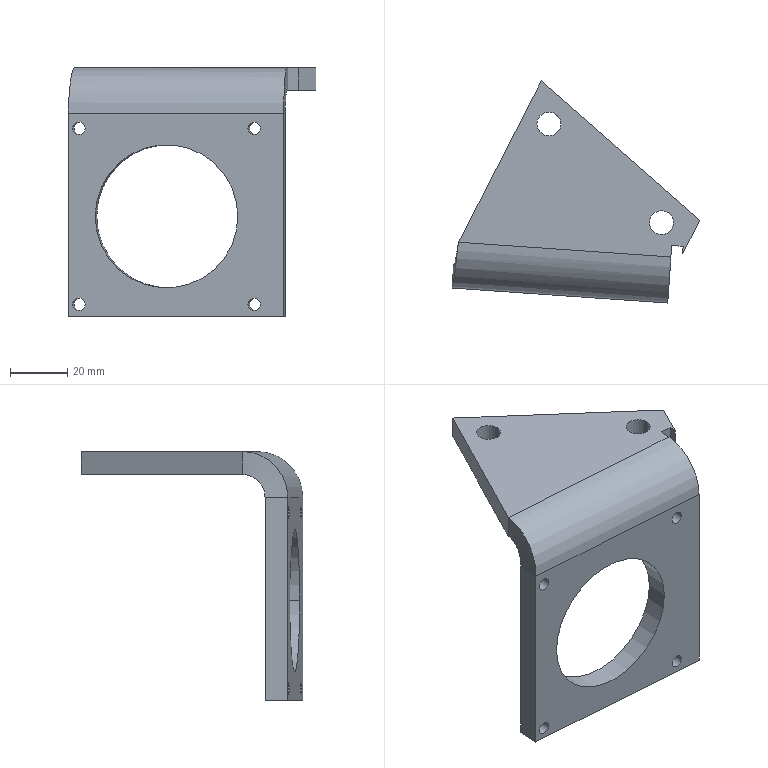Part | SolidWorks | features Cut 1, EdgeFlange 1, FlatPattern 1, ICE 1, SMBaseFlange 1, SheetMetal 1 | 1 solid | 31 faces | box 86.705 x 77.475 x 87.001 mm | volume 59436 mm3 | cylinder 16 | plane 14 | spline 1 | commonest cylinder face diameters 4.4 x8 8.382 x2 8.4 x2 50 x2 16 x1 32 x1
STEP:
#1=CARTESIAN_POINT('',(-134.069,-149.706,-52.));
#2=VERTEX_POINT('',#1);
#3=CARTESIAN_POINT('',(-183.95,-146.258,-52.));
#4=VERTEX_POINT('',#3);
#5=CARTESIAN_POINT('',(-159.009,-147.982,-52.));
#6=DIRECTION('',(0.06897,0.9976,0.));
#7=DIRECTION('',(-0.9976,0.06897,0.));
#8=AXIS2_PLACEMENT_3D('',#5,#6,#7);
#9=CIRCLE('',#8,25.);
#10=EDGE_CURVE('',#2,#4,#9,.T.);
#11=ORIENTED_EDGE('',*,*,#10,.F.);
#12=CARTESIAN_POINT('',(-133.517,-141.725,-52.));
#13=VERTEX_POINT('',#12);
#14=CARTESIAN_POINT('',(-134.207,-151.701,-52.));
#15=DIRECTION('',(0.06897,0.9976,0.));
#16=VECTOR('',#15,1000.);
#17=LINE('',#14,#16);
#18=EDGE_CURVE('',#2,#13,#17,.T.);
#19=ORIENTED_EDGE('',*,*,#18,.T.);
#20=CARTESIAN_POINT('',(-183.398,-138.277,-52.));
#21=VERTEX_POINT('',#20);
#22=CARTESIAN_POINT('',(-158.458,-140.001,-52.));
#23=DIRECTION('',(0.06897,0.9976,0.));
#24=DIRECTION('',(-0.9976,0.06897,0.));
#25=AXIS2_PLACEMENT_3D('',#22,#23,#24);
#26=CIRCLE('',#25,25.);
#27=EDGE_CURVE('',#13,#21,#26,.T.);
#28=ORIENTED_EDGE('',*,*,#27,.T.);
#29=CARTESIAN_POINT('',(-184.088,-148.253,-52.));
#30=DIRECTION('',(0.06897,0.9976,0.));
#31=VECTOR('',#30,1000.);
#32=LINE('',#29,#31);
#33=EDGE_CURVE('',#4,#21,#32,.T.);
#34=ORIENTED_EDGE('',*,*,#33,.F.);
#35=EDGE_LOOP('',(#11,#19,#28,#34));
#36=FACE_OUTER_BOUND('',#35,.T.);
#37=CARTESIAN_POINT('',(-159.147,-149.977,-52.));
#38=DIRECTION('',(0.06897,0.9976,0.));
#39=DIRECTION('',(-0.9976,0.06897,0.));
#40=AXIS2_PLACEMENT_3D('',#37,#38,#39);
#41=CYLINDRICAL_SURFACE('',#40,25.);
#42=ADVANCED_FACE('',(#36),#41,.F.);
#43=CARTESIAN_POINT('',(-126.136,-150.255,-82.75));
#44=VERTEX_POINT('',#43);
#45=CARTESIAN_POINT('',(-130.525,-149.951,-82.75));
#46=VERTEX_POINT('',#45);
#47=CARTESIAN_POINT('',(-128.33,-150.103,-82.75));
#48=DIRECTION('',(0.06897,0.9976,0.));
#49=DIRECTION('',(-0.9976,0.06897,0.));
#50=AXIS2_PLACEMENT_3D('',#47,#48,#49);
#51=CIRCLE('',#50,2.2);
#52=EDGE_CURVE('',#44,#46,#51,.T.);
#53=ORIENTED_EDGE('',*,*,#52,.F.);
#54=CARTESIAN_POINT('',(-125.584,-142.274,-82.75));
#55=VERTEX_POINT('',#54);
#56=CARTESIAN_POINT('',(-128.515,-184.673,-82.75));
#57=DIRECTION('',(0.06897,0.9976,0.));
#58=VECTOR('',#57,1000.);
#59=LINE('',#56,#58);
#60=EDGE_CURVE('',#44,#55,#59,.T.);
#61=ORIENTED_EDGE('',*,*,#60,.T.);
#62=CARTESIAN_POINT('',(-129.973,-141.97,-82.75));
#63=VERTEX_POINT('',#62);
#64=CARTESIAN_POINT('',(-127.779,-142.122,-82.75));
#65=DIRECTION('',(0.06897,0.9976,0.));
#66=DIRECTION('',(-0.9976,0.06897,0.));
#67=AXIS2_PLACEMENT_3D('',#64,#65,#66);
#68=CIRCLE('',#67,2.2);
#69=EDGE_CURVE('',#55,#63,#68,.T.);
#70=ORIENTED_EDGE('',*,*,#69,.T.);
#71=CARTESIAN_POINT('',(-132.905,-184.369,-82.75));
#72=DIRECTION('',(0.06897,0.9976,0.));
#73=VECTOR('',#72,1000.);
#74=LINE('',#71,#73);
#75=EDGE_CURVE('',#46,#63,#74,.T.);
#76=ORIENTED_EDGE('',*,*,#75,.F.);
#77=EDGE_LOOP('',(#53,#61,#70,#76));
#78=FACE_OUTER_BOUND('',#77,.T.);
#79=CARTESIAN_POINT('',(-130.71,-184.521,-82.75));
#80=DIRECTION('',(0.06897,0.9976,0.));
#81=DIRECTION('',(-0.9976,0.06897,0.));
#82=AXIS2_PLACEMENT_3D('',#79,#80,#81);
#83=CYLINDRICAL_SURFACE('',#82,2.2);
#84=ADVANCED_FACE('',(#78),#83,.F.);
#85=CARTESIAN_POINT('',(-187.489,-146.013,-82.75));
#86=VERTEX_POINT('',#85);
#87=CARTESIAN_POINT('',(-191.879,-145.709,-82.75));
#88=VERTEX_POINT('',#87);
#89=CARTESIAN_POINT('',(-189.684,-145.861,-82.75));
#90=DIRECTION('',(0.06897,0.9976,0.));
#91=DIRECTION('',(-0.9976,0.06897,0.));
#92=AXIS2_PLACEMENT_3D('',#89,#90,#91);
#93=CIRCLE('',#92,2.2);
#94=EDGE_CURVE('',#86,#88,#93,.T.);
#95=ORIENTED_EDGE('',*,*,#94,.F.);
#96=CARTESIAN_POINT('',(-186.937,-138.032,-82.75));
#97=VERTEX_POINT('',#96);
#98=CARTESIAN_POINT('',(-189.869,-180.431,-82.75));
#99=DIRECTION('',(0.06897,0.9976,0.));
#100=VECTOR('',#99,1000.);
#101=LINE('',#98,#100);
#102=EDGE_CURVE('',#86,#97,#101,.T.);
#103=ORIENTED_EDGE('',*,*,#102,.T.);
#104=CARTESIAN_POINT('',(-191.327,-137.729,-82.75));
#105=VERTEX_POINT('',#104);
#106=CARTESIAN_POINT('',(-189.132,-137.88,-82.75));
#107=DIRECTION('',(0.06897,0.9976,0.));
#108=DIRECTION('',(-0.9976,0.06897,0.));
#109=AXIS2_PLACEMENT_3D('',#106,#107,#108);
#110=CIRCLE('',#109,2.2);
#111=EDGE_CURVE('',#97,#105,#110,.T.);
#112=ORIENTED_EDGE('',*,*,#111,.T.);
#113=CARTESIAN_POINT('',(-194.258,-180.127,-82.75));
#114=DIRECTION('',(0.06897,0.9976,0.));
#115=VECTOR('',#114,1000.);
#116=LINE('',#113,#115);
#117=EDGE_CURVE('',#88,#105,#116,.T.);
#118=ORIENTED_EDGE('',*,*,#117,.F.);
#119=EDGE_LOOP('',(#95,#103,#112,#118));
#120=FACE_OUTER_BOUND('',#119,.T.);
#121=CARTESIAN_POINT('',(-192.063,-180.279,-82.75));
#122=DIRECTION('',(0.06897,0.9976,0.));
#123=DIRECTION('',(-0.9976,0.06897,0.));
#124=AXIS2_PLACEMENT_3D('',#121,#122,#123);
#125=CYLINDRICAL_SURFACE('',#124,2.2);
#126=ADVANCED_FACE('',(#120),#125,.F.);
#127=CARTESIAN_POINT('',(-187.489,-146.013,-21.25));
#128=VERTEX_POINT('',#127);
#129=CARTESIAN_POINT('',(-191.879,-145.709,-21.25));
#130=VERTEX_POINT('',#129);
#131=CARTESIAN_POINT('',(-189.684,-145.861,-21.25));
#132=DIRECTION('',(0.06897,0.9976,0.));
#133=DIRECTION('',(-0.9976,0.06897,0.));
#134=AXIS2_PLACEMENT_3D('',#131,#132,#133);
#135=CIRCLE('',#134,2.2);
#136=EDGE_CURVE('',#128,#130,#135,.T.);
#137=ORIENTED_EDGE('',*,*,#136,.F.);
#138=CARTESIAN_POINT('',(-186.937,-138.032,-21.25));
#139=VERTEX_POINT('',#138);
#140=CARTESIAN_POINT('',(-189.869,-180.431,-21.25));
#141=DIRECTION('',(0.06897,0.9976,0.));
#142=VECTOR('',#141,1000.);
#143=LINE('',#140,#142);
#144=EDGE_CURVE('',#128,#139,#143,.T.);
#145=ORIENTED_EDGE('',*,*,#144,.T.);
#146=CARTESIAN_POINT('',(-191.327,-137.729,-21.25));
#147=VERTEX_POINT('',#146);
#148=CARTESIAN_POINT('',(-189.132,-137.88,-21.25));
#149=DIRECTION('',(0.06897,0.9976,0.));
#150=DIRECTION('',(-0.9976,0.06897,0.));
#151=AXIS2_PLACEMENT_3D('',#148,#149,#150);
#152=CIRCLE('',#151,2.2);
#153=EDGE_CURVE('',#139,#147,#152,.T.);
#154=ORIENTED_EDGE('',*,*,#153,.T.);
#155=CARTESIAN_POINT('',(-194.258,-180.127,-21.25));
#156=DIRECTION('',(0.06897,0.9976,0.));
#157=VECTOR('',#156,1000.);
#158=LINE('',#155,#157);
#159=EDGE_CURVE('',#130,#147,#158,.T.);
#160=ORIENTED_EDGE('',*,*,#159,.F.);
#161=EDGE_LOOP('',(#137,#145,#154,#160));
#162=FACE_OUTER_BOUND('',#161,.T.);
#163=CARTESIAN_POINT('',(-192.063,-180.279,-21.25));
#164=DIRECTION('',(0.06897,0.9976,0.));
#165=DIRECTION('',(-0.9976,0.06897,0.));
#166=AXIS2_PLACEMENT_3D('',#163,#164,#165);
#167=CYLINDRICAL_SURFACE('',#166,2.2);
#168=ADVANCED_FACE('',(#162),#167,.F.);
#169=CARTESIAN_POINT('',(-126.136,-150.255,-21.25));
#170=VERTEX_POINT('',#169);
#171=CARTESIAN_POINT('',(-130.525,-149.951,-21.25));
#172=VERTEX_POINT('',#171);
#173=CARTESIAN_POINT('',(-128.33,-150.103,-21.25));
#174=DIRECTION('',(0.06897,0.9976,0.));
#175=DIRECTION('',(-0.9976,0.06897,0.));
#176=AXIS2_PLACEMENT_3D('',#173,#174,#175);
#177=CIRCLE('',#176,2.2);
#178=EDGE_CURVE('',#170,#172,#177,.T.);
#179=ORIENTED_EDGE('',*,*,#178,.F.);
#180=CARTESIAN_POINT('',(-125.584,-142.274,-21.25));
#181=VERTEX_POINT('',#180);
#182=CARTESIAN_POINT('',(-128.515,-184.673,-21.25));
#183=DIRECTION('',(0.06897,0.9976,0.));
#184=VECTOR('',#183,1000.);
#185=LINE('',#182,#184);
#186=EDGE_CURVE('',#170,#181,#185,.T.);
#187=ORIENTED_EDGE('',*,*,#186,.T.);
#188=CARTESIAN_POINT('',(-129.973,-141.97,-21.25));
#189=VERTEX_POINT('',#188);
#190=CARTESIAN_POINT('',(-127.779,-142.122,-21.25));
#191=DIRECTION('',(0.06897,0.9976,0.));
#192=DIRECTION('',(-0.9976,0.06897,0.));
#193=AXIS2_PLACEMENT_3D('',#190,#191,#192);
#194=CIRCLE('',#193,2.2);
#195=EDGE_CURVE('',#181,#189,#194,.T.);
#196=ORIENTED_EDGE('',*,*,#195,.T.);
#197=CARTESIAN_POINT('',(-132.905,-184.369,-21.25));
#198=DIRECTION('',(0.06897,0.9976,0.));
#199=VECTOR('',#198,1000.);
#200=LINE('',#197,#199);
#201=EDGE_CURVE('',#172,#189,#200,.T.);
#202=ORIENTED_EDGE('',*,*,#201,.F.);
#203=EDGE_LOOP('',(#179,#187,#196,#202));
#204=FACE_OUTER_BOUND('',#203,.T.);
#205=CARTESIAN_POINT('',(-130.71,-184.521,-21.25));
#206=DIRECTION('',(0.06897,0.9976,0.));
#207=DIRECTION('',(-0.9976,0.06897,0.));
#208=AXIS2_PLACEMENT_3D('',#205,#206,#207);
#209=CYLINDRICAL_SURFACE('',#208,2.2);
#210=ADVANCED_FACE('',(#204),#209,.F.);
#211=CARTESIAN_POINT('',(-124.39,-122.853,-8.));
#212=VERTEX_POINT('',#211);
#213=CARTESIAN_POINT('',(-115.99,-122.853,-8.));
#214=VERTEX_POINT('',#213);
#215=CARTESIAN_POINT('',(-120.19,-122.853,-8.));
#216=DIRECTION('',(0.,0.,1.));
#217=DIRECTION('',(-1.,0.,0.));
#218=AXIS2_PLACEMENT_3D('',#215,#216,#217);
#219=CIRCLE('',#218,4.2);
#220=EDGE_CURVE('',#212,#214,#219,.T.);
#221=ORIENTED_EDGE('',*,*,#220,.F.);
#222=CARTESIAN_POINT('',(-124.39,-122.853,0.));
#223=VERTEX_POINT('',#222);
#224=CARTESIAN_POINT('',(-124.39,-122.853,-8.));
#225=DIRECTION('',(0.,0.,1.));
#226=VECTOR('',#225,1000.);
#227=LINE('',#224,#226);
#228=EDGE_CURVE('',#212,#223,#227,.T.);
#229=ORIENTED_EDGE('',*,*,#228,.T.);
#230=CARTESIAN_POINT('',(-115.99,-122.853,0.));
#231=VERTEX_POINT('',#230);
#232=CARTESIAN_POINT('',(-120.19,-122.853,0.));
#233=DIRECTION('',(0.,0.,1.));
#234=DIRECTION('',(-1.,0.,0.));
#235=AXIS2_PLACEMENT_3D('',#232,#233,#234);
#236=CIRCLE('',#235,4.2);
#237=EDGE_CURVE('',#223,#231,#236,.T.);
#238=ORIENTED_EDGE('',*,*,#237,.T.);
#239=CARTESIAN_POINT('',(-115.99,-122.853,-8.));
#240=DIRECTION('',(0.,0.,1.));
#241=VECTOR('',#240,1000.);
#242=LINE('',#239,#241);
#243=EDGE_CURVE('',#214,#231,#242,.T.);
#244=ORIENTED_EDGE('',*,*,#243,.F.);
#245=EDGE_LOOP('',(#221,#229,#238,#244));
#246=FACE_OUTER_BOUND('',#245,.T.);
#247=CARTESIAN_POINT('',(-120.19,-122.853,-8.));
#248=DIRECTION('',(0.,0.,1.));
#249=DIRECTION('',(1.,0.,0.));
#250=AXIS2_PLACEMENT_3D('',#247,#248,#249);
#251=CYLINDRICAL_SURFACE('',#250,4.2);
#252=ADVANCED_FACE('',(#246),#251,.F.);
#253=CARTESIAN_POINT('',(-163.77,-88.351,-8.));
#254=VERTEX_POINT('',#253);
#255=CARTESIAN_POINT('',(-155.388,-88.351,-8.));
#256=VERTEX_POINT('',#255);
#257=CARTESIAN_POINT('',(-159.579,-88.351,-8.));
#258=DIRECTION('',(0.,0.,1.));
#259=DIRECTION('',(-1.,0.,0.));
#260=AXIS2_PLACEMENT_3D('',#257,#258,#259);
#261=CIRCLE('',#260,4.191);
#262=EDGE_CURVE('',#254,#256,#261,.T.);
#263=ORIENTED_EDGE('',*,*,#262,.F.);
#264=CARTESIAN_POINT('',(-163.77,-88.351,0.));
#265=VERTEX_POINT('',#264);
#266=CARTESIAN_POINT('',(-163.77,-88.351,-8.));
#267=DIRECTION('',(0.,0.,1.));
#268=VECTOR('',#267,1000.);
#269=LINE('',#266,#268);
#270=EDGE_CURVE('',#254,#265,#269,.T.);
#271=ORIENTED_EDGE('',*,*,#270,.T.);
#272=CARTESIAN_POINT('',(-155.388,-88.351,0.));
#273=VERTEX_POINT('',#272);
#274=CARTESIAN_POINT('',(-159.579,-88.351,0.));
#275=DIRECTION('',(0.,0.,1.));
#276=DIRECTION('',(-1.,0.,0.));
#277=AXIS2_PLACEMENT_3D('',#274,#275,#276);
#278=CIRCLE('',#277,4.191);
#279=EDGE_CURVE('',#265,#273,#278,.T.);
#280=ORIENTED_EDGE('',*,*,#279,.T.);
#281=CARTESIAN_POINT('',(-155.388,-88.351,-8.));
#282=DIRECTION('',(0.,0.,1.));
#283=VECTOR('',#282,1000.);
#284=LINE('',#281,#283);
#285=EDGE_CURVE('',#256,#273,#284,.T.);
#286=ORIENTED_EDGE('',*,*,#285,.F.);
#287=EDGE_LOOP('',(#263,#271,#280,#286));
#288=FACE_OUTER_BOUND('',#287,.T.);
#289=CARTESIAN_POINT('',(-159.579,-88.351,-8.));
#290=DIRECTION('',(0.,0.,1.));
#291=DIRECTION('',(1.,0.,0.));
#292=AXIS2_PLACEMENT_3D('',#289,#290,#291);
#293=CYLINDRICAL_SURFACE('',#292,4.191);
#294=ADVANCED_FACE('',(#288),#293,.F.);
#295=CARTESIAN_POINT('',(-112.832,-133.812,0.));
#296=VERTEX_POINT('',#295);
#297=CARTESIAN_POINT('',(-106.749,-121.964,0.));
#298=VERTEX_POINT('',#297);
#299=CARTESIAN_POINT('',(-113.489,-135.091,0.));
#300=DIRECTION('',(0.4568,0.8896,0.));
#301=VECTOR('',#300,1000.);
#302=LINE('',#299,#301);
#303=EDGE_CURVE('',#296,#298,#302,.T.);
#304=ORIENTED_EDGE('',*,*,#303,.F.);
#305=CARTESIAN_POINT('',(-112.832,-133.812,-8.));
#306=VERTEX_POINT('',#305);
#307=CARTESIAN_POINT('',(-112.832,-133.812,-8.));
#308=DIRECTION('',(0.,0.,-1.));
#309=VECTOR('',#308,1000.);
#310=LINE('',#307,#309);
#311=EDGE_CURVE('',#296,#306,#310,.T.);
#312=ORIENTED_EDGE('',*,*,#311,.T.);
#313=CARTESIAN_POINT('',(-106.749,-121.964,-8.));
#314=VERTEX_POINT('',#313);
#315=CARTESIAN_POINT('',(-113.489,-135.091,-8.));
#316=DIRECTION('',(0.4568,0.8896,0.));
#317=VECTOR('',#316,1000.);
#318=LINE('',#315,#317);
#319=EDGE_CURVE('',#306,#314,#318,.T.);
#320=ORIENTED_EDGE('',*,*,#319,.T.);
#321=CARTESIAN_POINT('',(-106.749,-121.964,-8.));
#322=DIRECTION('',(0.,0.,1.));
#323=VECTOR('',#322,1000.);
#324=LINE('',#321,#323);
#325=EDGE_CURVE('',#314,#298,#324,.T.);
#326=ORIENTED_EDGE('',*,*,#325,.T.);
#327=EDGE_LOOP('',(#304,#312,#320,#326));
#328=FACE_OUTER_BOUND('',#327,.T.);
#329=CARTESIAN_POINT('',(-113.489,-135.091,-8.));
#330=DIRECTION('',(0.8896,-0.4568,0.));
#331=DIRECTION('',(0.4568,0.8896,0.));
#332=AXIS2_PLACEMENT_3D('',#329,#330,#331);
#333=PLANE('',#332);
#334=ADVANCED_FACE('',(#328),#333,.T.);
#335=CARTESIAN_POINT('',(-120.19,-122.853,-8.));
#336=DIRECTION('',(0.,0.,1.));
#337=DIRECTION('',(-1.,0.,0.));
#338=AXIS2_PLACEMENT_3D('',#335,#336,#337);
#339=CIRCLE('',#338,4.2);
#340=EDGE_CURVE('',#214,#212,#339,.T.);
#341=ORIENTED_EDGE('',*,*,#340,.T.);
#342=ORIENTED_EDGE('',*,*,#220,.T.);
#343=EDGE_LOOP('',(#341,#342));
#344=FACE_BOUND('',#343,.T.);
#345=CARTESIAN_POINT('',(-159.579,-88.351,-8.));
#346=DIRECTION('',(0.,0.,1.));
#347=DIRECTION('',(-1.,0.,0.));
#348=AXIS2_PLACEMENT_3D('',#345,#346,#347);
#349=CIRCLE('',#348,4.191);
#350=EDGE_CURVE('',#256,#254,#349,.T.);
#351=ORIENTED_EDGE('',*,*,#350,.T.);
#352=ORIENTED_EDGE('',*,*,#262,.T.);
#353=EDGE_LOOP('',(#351,#352));
#354=FACE_BOUND('',#353,.T.);
#355=CARTESIAN_POINT('',(-191.208,-129.718,-8.));
#356=VERTEX_POINT('',#355);
#357=CARTESIAN_POINT('',(-116.914,-134.854,-8.));
#358=VERTEX_POINT('',#357);
#359=CARTESIAN_POINT('',(-192.35,-129.639,-8.));
#360=DIRECTION('',(0.9976,-0.06897,0.));
#361=VECTOR('',#360,1000.);
#362=LINE('',#359,#361);
#363=EDGE_CURVE('',#356,#358,#362,.T.);
#364=ORIENTED_EDGE('',*,*,#363,.F.);
#365=CARTESIAN_POINT('',(-162.259,-73.341,-8.));
#366=VERTEX_POINT('',#365);
#367=CARTESIAN_POINT('',(-162.259,-73.341,-8.));
#368=DIRECTION('',(-0.4568,-0.8896,0.));
#369=VECTOR('',#368,1000.);
#370=LINE('',#367,#369);
#371=EDGE_CURVE('',#366,#356,#370,.T.);
#372=ORIENTED_EDGE('',*,*,#371,.F.);
#373=CARTESIAN_POINT('',(-106.749,-121.964,-8.));
#374=DIRECTION('',(-0.7522,0.6589,0.));
#375=VECTOR('',#374,1000.);
#376=LINE('',#373,#375);
#377=EDGE_CURVE('',#314,#366,#376,.T.);
#378=ORIENTED_EDGE('',*,*,#377,.F.);
#379=ORIENTED_EDGE('',*,*,#319,.F.);
#380=CARTESIAN_POINT('',(-112.647,-131.139,-8.));
#381=VERTEX_POINT('',#380);
#382=CARTESIAN_POINT('',(-112.647,-131.139,-8.));
#383=DIRECTION('',(-0.06897,-0.9976,0.));
#384=VECTOR('',#383,1000.);
#385=LINE('',#382,#384);
#386=EDGE_CURVE('',#381,#306,#385,.T.);
#387=ORIENTED_EDGE('',*,*,#386,.F.);
#388=CARTESIAN_POINT('',(-116.638,-130.864,-8.));
#389=VERTEX_POINT('',#388);
#390=CARTESIAN_POINT('',(-116.638,-130.864,-8.));
#391=DIRECTION('',(0.9976,-0.06897,0.));
#392=VECTOR('',#391,1000.);
#393=LINE('',#390,#392);
#394=EDGE_CURVE('',#389,#381,#393,.T.);
#395=ORIENTED_EDGE('',*,*,#394,.F.);
#396=CARTESIAN_POINT('',(-116.914,-134.854,-8.));
#397=DIRECTION('',(0.06897,0.9976,0.));
#398=VECTOR('',#397,1000.);
#399=LINE('',#396,#398);
#400=EDGE_CURVE('',#358,#389,#399,.T.);
#401=ORIENTED_EDGE('',*,*,#400,.F.);
#402=EDGE_LOOP('',(#364,#372,#378,#379,#387,#395,#401));
#403=FACE_OUTER_BOUND('',#402,.T.);
#404=CARTESIAN_POINT('',(-192.063,-133.805,-8.));
#405=DIRECTION('',(0.,0.,1.));
#406=DIRECTION('',(1.,0.,0.));
#407=AXIS2_PLACEMENT_3D('',#404,#405,#406);
#408=PLANE('',#407);
#409=ADVANCED_FACE('',(#344,#354,#403),#408,.F.);
#410=CARTESIAN_POINT('',(-120.19,-122.853,0.));
#411=DIRECTION('',(0.,0.,1.));
#412=DIRECTION('',(-1.,0.,0.));
#413=AXIS2_PLACEMENT_3D('',#410,#411,#412);
#414=CIRCLE('',#413,4.2);
#415=EDGE_CURVE('',#231,#223,#414,.T.);
#416=ORIENTED_EDGE('',*,*,#415,.F.);
#417=ORIENTED_EDGE('',*,*,#237,.F.);
#418=EDGE_LOOP('',(#416,#417));
#419=FACE_BOUND('',#418,.T.);
#420=CARTESIAN_POINT('',(-159.579,-88.351,0.));
#421=DIRECTION('',(0.,0.,1.));
#422=DIRECTION('',(-1.,0.,0.));
#423=AXIS2_PLACEMENT_3D('',#420,#421,#422);
#424=CIRCLE('',#423,4.191);
#425=EDGE_CURVE('',#273,#265,#424,.T.);
#426=ORIENTED_EDGE('',*,*,#425,.F.);
#427=ORIENTED_EDGE('',*,*,#279,.F.);
#428=EDGE_LOOP('',(#426,#427));
#429=FACE_BOUND('',#428,.T.);
#430=CARTESIAN_POINT('',(-162.259,-73.341,0.));
#431=VERTEX_POINT('',#430);
#432=CARTESIAN_POINT('',(-191.208,-129.718,0.0005));
#433=VERTEX_POINT('',#432);
#434=CARTESIAN_POINT('',(-162.259,-73.341,0.));
#435=DIRECTION('',(-0.4568,-0.8896,0.));
#436=VECTOR('',#435,1000.);
#437=LINE('',#434,#436);
#438=EDGE_CURVE('',#431,#433,#437,.T.);
#439=ORIENTED_EDGE('',*,*,#438,.T.);
#440=CARTESIAN_POINT('',(-116.914,-134.854,0.));
#441=VERTEX_POINT('',#440);
#442=CARTESIAN_POINT('',(-192.35,-129.639,0.));
#443=DIRECTION('',(0.9976,-0.06897,0.));
#444=VECTOR('',#443,1000.);
#445=LINE('',#442,#444);
#446=EDGE_CURVE('',#433,#441,#445,.T.);
#447=ORIENTED_EDGE('',*,*,#446,.T.);
#448=CARTESIAN_POINT('',(-116.638,-130.864,0.));
#449=VERTEX_POINT('',#448);
#450=CARTESIAN_POINT('',(-117.199,-138.981,0.));
#451=DIRECTION('',(0.06897,0.9976,0.));
#452=VECTOR('',#451,1000.);
#453=LINE('',#450,#452);
#454=EDGE_CURVE('',#441,#449,#453,.T.);
#455=ORIENTED_EDGE('',*,*,#454,.T.);
#456=CARTESIAN_POINT('',(-112.647,-131.139,0.));
#457=VERTEX_POINT('',#456);
#458=CARTESIAN_POINT('',(-191.502,-125.688,0.));
#459=DIRECTION('',(0.9976,-0.06897,0.));
#460=VECTOR('',#459,1000.);
#461=LINE('',#458,#460);
#462=EDGE_CURVE('',#449,#457,#461,.T.);
#463=ORIENTED_EDGE('',*,*,#462,.T.);
#464=CARTESIAN_POINT('',(-113.209,-139.257,0.));
#465=DIRECTION('',(-0.06897,-0.9976,0.));
#466=VECTOR('',#465,1000.);
#467=LINE('',#464,#466);
#468=EDGE_CURVE('',#457,#296,#467,.T.);
#469=ORIENTED_EDGE('',*,*,#468,.T.);
#470=ORIENTED_EDGE('',*,*,#303,.T.);
#471=CARTESIAN_POINT('',(-106.749,-121.964,0.));
#472=DIRECTION('',(-0.7522,0.6589,0.));
#473=VECTOR('',#472,1000.);
#474=LINE('',#471,#473);
#475=EDGE_CURVE('',#298,#431,#474,.T.);
#476=ORIENTED_EDGE('',*,*,#475,.T.);
#477=EDGE_LOOP('',(#439,#447,#455,#463,#469,#470,#476));
#478=FACE_OUTER_BOUND('',#477,.T.);
#479=CARTESIAN_POINT('',(-192.063,-133.805,0.));
#480=DIRECTION('',(0.,0.,1.));
#481=DIRECTION('',(1.,0.,0.));
#482=AXIS2_PLACEMENT_3D('',#479,#480,#481);
#483=PLANE('',#482);
#484=ADVANCED_FACE('',(#419,#429,#478),#483,.T.);
#485=ORIENTED_EDGE('',*,*,#438,.F.);
#486=CARTESIAN_POINT('',(-162.259,-73.341,-8.));
#487=DIRECTION('',(0.,0.,1.));
#488=VECTOR('',#487,1000.);
#489=LINE('',#486,#488);
#490=EDGE_CURVE('',#366,#431,#489,.T.);
#491=ORIENTED_EDGE('',*,*,#490,.F.);
#492=ORIENTED_EDGE('',*,*,#371,.T.);
#493=CARTESIAN_POINT('',(-191.208,-129.718,-8.));
#494=DIRECTION('',(0.,0.,1.));
#495=VECTOR('',#494,1000.);
#496=LINE('',#493,#495);
#497=EDGE_CURVE('',#356,#433,#496,.T.);
#498=ORIENTED_EDGE('',*,*,#497,.T.);
#499=EDGE_LOOP('',(#485,#491,#492,#498));
#500=FACE_OUTER_BOUND('',#499,.T.);
#501=CARTESIAN_POINT('',(-162.259,-73.341,-8.));
#502=DIRECTION('',(-0.8896,0.4568,0.));
#503=DIRECTION('',(-0.4568,-0.8896,0.));
#504=AXIS2_PLACEMENT_3D('',#501,#502,#503);
#505=PLANE('',#504);
#506=ADVANCED_FACE('',(#500),#505,.T.);
#507=ORIENTED_EDGE('',*,*,#475,.F.);
#508=ORIENTED_EDGE('',*,*,#325,.F.);
#509=ORIENTED_EDGE('',*,*,#377,.T.);
#510=ORIENTED_EDGE('',*,*,#490,.T.);
#511=EDGE_LOOP('',(#507,#508,#509,#510));
#512=FACE_OUTER_BOUND('',#511,.T.);
#513=CARTESIAN_POINT('',(-106.749,-121.964,-8.));
#514=DIRECTION('',(0.6589,0.7522,0.));
#515=DIRECTION('',(-0.7522,0.6589,0.));
#516=AXIS2_PLACEMENT_3D('',#513,#514,#515);
#517=PLANE('',#516);
#518=ADVANCED_FACE('',(#512),#517,.T.);
#519=ORIENTED_EDGE('',*,*,#270,.F.);
#520=ORIENTED_EDGE('',*,*,#350,.F.);
#521=ORIENTED_EDGE('',*,*,#285,.T.);
#522=ORIENTED_EDGE('',*,*,#425,.T.);
#523=EDGE_LOOP('',(#519,#520,#521,#522));
#524=FACE_OUTER_BOUND('',#523,.T.);
#525=CARTESIAN_POINT('',(-159.579,-88.351,-8.));
#526=DIRECTION('',(0.,0.,1.));
#527=DIRECTION('',(1.,0.,0.));
#528=AXIS2_PLACEMENT_3D('',#525,#526,#527);
#529=CYLINDRICAL_SURFACE('',#528,4.191);
#530=ADVANCED_FACE('',(#524),#529,.F.);
#531=ORIENTED_EDGE('',*,*,#228,.F.);
#532=ORIENTED_EDGE('',*,*,#340,.F.);
#533=ORIENTED_EDGE('',*,*,#243,.T.);
#534=ORIENTED_EDGE('',*,*,#415,.T.);
#535=EDGE_LOOP('',(#531,#532,#533,#534));
#536=FACE_OUTER_BOUND('',#535,.T.);
#537=CARTESIAN_POINT('',(-120.19,-122.853,-8.));
#538=DIRECTION('',(0.,0.,1.));
#539=DIRECTION('',(1.,0.,0.));
#540=AXIS2_PLACEMENT_3D('',#537,#538,#539);
#541=CYLINDRICAL_SURFACE('',#540,4.2);
#542=ADVANCED_FACE('',(#536),#541,.F.);
#543=ORIENTED_EDGE('',*,*,#454,.F.);
#544=CARTESIAN_POINT('',(-116.914,-134.854,-8.));
#545=DIRECTION('',(0.,0.,1.));
#546=VECTOR('',#545,1000.);
#547=LINE('',#544,#546);
#548=EDGE_CURVE('',#358,#441,#547,.T.);
#549=ORIENTED_EDGE('',*,*,#548,.F.);
#550=ORIENTED_EDGE('',*,*,#400,.T.);
#551=CARTESIAN_POINT('',(-116.638,-130.864,-8.));
#552=DIRECTION('',(0.,0.,1.));
#553=VECTOR('',#552,1000.);
#554=LINE('',#551,#553);
#555=EDGE_CURVE('',#389,#449,#554,.T.);
#556=ORIENTED_EDGE('',*,*,#555,.T.);
#557=EDGE_LOOP('',(#543,#549,#550,#556));
#558=FACE_OUTER_BOUND('',#557,.T.);
#559=CARTESIAN_POINT('',(-116.914,-134.854,-8.));
#560=DIRECTION('',(0.9976,-0.06897,0.));
#561=DIRECTION('',(0.06897,0.9976,0.));
#562=AXIS2_PLACEMENT_3D('',#559,#560,#561);
#563=PLANE('',#562);
#564=ADVANCED_FACE('',(#558),#563,.T.);
#565=ORIENTED_EDGE('',*,*,#462,.F.);
#566=ORIENTED_EDGE('',*,*,#555,.F.);
#567=ORIENTED_EDGE('',*,*,#394,.T.);
#568=CARTESIAN_POINT('',(-112.647,-131.139,-8.));
#569=DIRECTION('',(0.,0.,1.));
#570=VECTOR('',#569,1000.);
#571=LINE('',#568,#570);
#572=EDGE_CURVE('',#381,#457,#571,.T.);
#573=ORIENTED_EDGE('',*,*,#572,.T.);
#574=EDGE_LOOP('',(#565,#566,#567,#573));
#575=FACE_OUTER_BOUND('',#574,.T.);
#576=CARTESIAN_POINT('',(-116.638,-130.864,-8.));
#577=DIRECTION('',(-0.06897,-0.9976,0.));
#578=DIRECTION('',(0.9976,-0.06897,0.));
#579=AXIS2_PLACEMENT_3D('',#576,#577,#578);
#580=PLANE('',#579);
#581=ADVANCED_FACE('',(#575),#580,.T.);
#582=ORIENTED_EDGE('',*,*,#311,.F.);
#583=ORIENTED_EDGE('',*,*,#468,.F.);
#584=ORIENTED_EDGE('',*,*,#572,.F.);
#585=ORIENTED_EDGE('',*,*,#386,.T.);
#586=EDGE_LOOP('',(#582,#583,#584,#585));
#587=FACE_OUTER_BOUND('',#586,.T.);
#588=CARTESIAN_POINT('',(-112.647,-131.139,-8.));
#589=DIRECTION('',(-0.9976,0.06897,0.));
#590=DIRECTION('',(-0.06897,-0.9976,0.));
#591=AXIS2_PLACEMENT_3D('',#588,#589,#590);
#592=PLANE('',#591);
#593=ADVANCED_FACE('',(#587),#592,.T.);
#594=CARTESIAN_POINT('',(-117.466,-142.835,-16.));
#595=VERTEX_POINT('',#594);
#596=CARTESIAN_POINT('',(-118.017,-150.816,-16.));
#597=VERTEX_POINT('',#596);
#598=CARTESIAN_POINT('',(-117.466,-142.835,-16.));
#599=DIRECTION('',(-0.06897,-0.9976,0.));
#600=VECTOR('',#599,1000.);
#601=LINE('',#598,#600);
#602=EDGE_CURVE('',#595,#597,#601,.T.);
#603=ORIENTED_EDGE('',*,*,#602,.F.);
#604=CARTESIAN_POINT('',(-116.914,-134.854,-16.));
#605=DIRECTION('',(0.9976,-0.06897,0.));
#606=DIRECTION('',(-0.06897,-0.9976,0.));
#607=AXIS2_PLACEMENT_3D('',#604,#605,#606);
#608=CIRCLE('',#607,8.);
#609=EDGE_CURVE('',#358,#595,#608,.T.);
#610=ORIENTED_EDGE('',*,*,#609,.F.);
#611=ORIENTED_EDGE('',*,*,#548,.T.);
#612=CARTESIAN_POINT('',(-116.914,-134.854,-16.));
#613=DIRECTION('',(0.9976,-0.06897,0.));
#614=DIRECTION('',(-0.06897,-0.9976,0.));
#615=AXIS2_PLACEMENT_3D('',#612,#613,#614);
#616=CIRCLE('',#615,16.);
#617=EDGE_CURVE('',#441,#597,#616,.T.);
#618=ORIENTED_EDGE('',*,*,#617,.T.);
#619=EDGE_LOOP('',(#603,#610,#611,#618));
#620=FACE_OUTER_BOUND('',#619,.T.);
#621=CARTESIAN_POINT('',(-116.914,-134.854,-16.));
#622=DIRECTION('',(0.9976,-0.06897,0.));
#623=DIRECTION('',(0.06897,0.9976,0.));
#624=AXIS2_PLACEMENT_3D('',#621,#622,#623);
#625=PLANE('',#624);
#626=ADVANCED_FACE('',(#620),#625,.T.);
#627=CARTESIAN_POINT('',(-192.901,-137.62,-16.));
#628=VERTEX_POINT('',#627);
#629=CARTESIAN_POINT('',(-192.901,-137.62,-16.));
#630=CARTESIAN_POINT('',(-192.853,-137.623,-15.472));
#631=CARTESIAN_POINT('',(-192.803,-137.575,-14.952));
#632=CARTESIAN_POINT('',(-192.721,-137.428,-14.186));
#633=CARTESIAN_POINT('',(-192.693,-137.366,-13.933));
#634=CARTESIAN_POINT('',(-192.635,-137.218,-13.43));
#635=CARTESIAN_POINT('',(-192.605,-137.13,-13.181));
#636=CARTESIAN_POINT('',(-192.512,-136.835,-12.454));
#637=CARTESIAN_POINT('',(-192.448,-136.593,-11.995));
#638=CARTESIAN_POINT('',(-192.314,-136.022,-11.126));
#639=CARTESIAN_POINT('',(-192.242,-135.688,-10.714));
#640=CARTESIAN_POINT('',(-192.097,-134.959,-9.976));
#641=CARTESIAN_POINT('',(-192.022,-134.561,-9.645));
#642=CARTESIAN_POINT('',(-191.905,-133.913,-9.207));
#643=CARTESIAN_POINT('',(-191.865,-133.688,-9.07));
#644=CARTESIAN_POINT('',(-191.786,-133.23,-8.823));
#645=CARTESIAN_POINT('',(-191.746,-132.997,-8.712));
#646=CARTESIAN_POINT('',(-191.625,-132.282,-8.412));
#647=CARTESIAN_POINT('',(-191.543,-131.784,-8.258));
#648=CARTESIAN_POINT('',(-191.376,-130.759,-8.052));
#649=CARTESIAN_POINT('',(-191.292,-130.241,-8.));
#650=CARTESIAN_POINT('',(-191.208,-129.718,-8.));
#651=B_SPLINE_CURVE_WITH_KNOTS('',3,(#629,#630,#631,#632,#633,#634,#635,#636,#637,#638,#639,#640,#641,#642,#643,#644,#645,#646,#647,#648,#649,#650),.UNSPECIFIED.,.F.,.F.,(4,2,2,2,2,2,2,2,2,2,4),(0.,0.001569,0.002353,0.003137,0.004706,0.006274,0.007843,0.008627,0.009412,0.01098,0.01255),.UNSPECIFIED.);
#652=EDGE_CURVE('',#628,#356,#651,.T.);
#653=ORIENTED_EDGE('',*,*,#652,.F.);
#654=CARTESIAN_POINT('',(-193.453,-145.601,-16.));
#655=VERTEX_POINT('',#654);
#656=CARTESIAN_POINT('',(-192.901,-137.62,-16.));
#657=DIRECTION('',(-0.06897,-0.9976,0.));
#658=VECTOR('',#657,1000.);
#659=LINE('',#656,#658);
#660=EDGE_CURVE('',#628,#655,#659,.T.);
#661=ORIENTED_EDGE('',*,*,#660,.T.);
#662=CARTESIAN_POINT('',(-193.453,-145.601,-16.));
#663=CARTESIAN_POINT('',(-193.405,-145.604,-14.944));
#664=CARTESIAN_POINT('',(-193.351,-145.504,-13.905));
#665=CARTESIAN_POINT('',(-193.259,-145.205,-12.372));
#666=CARTESIAN_POINT('',(-193.226,-145.08,-11.865));
#667=CARTESIAN_POINT('',(-193.158,-144.78,-10.861));
#668=CARTESIAN_POINT('',(-193.121,-144.604,-10.361));
#669=CARTESIAN_POINT('',(-193.008,-144.009,-8.909));
#670=CARTESIAN_POINT('',(-192.927,-143.522,-7.99));
#671=CARTESIAN_POINT('',(-192.796,-142.659,-6.686));
#672=CARTESIAN_POINT('',(-192.751,-142.348,-6.263));
#673=CARTESIAN_POINT('',(-192.657,-141.684,-5.447));
#674=CARTESIAN_POINT('',(-192.609,-141.335,-5.059));
#675=CARTESIAN_POINT('',(-192.461,-140.237,-3.952));
#676=CARTESIAN_POINT('',(-192.359,-139.437,-3.29));
#677=CARTESIAN_POINT('',(-192.197,-138.135,-2.413));
#678=CARTESIAN_POINT('',(-192.141,-137.684,-2.14));
#679=CARTESIAN_POINT('',(-192.03,-136.766,-1.646));
#680=CARTESIAN_POINT('',(-191.974,-136.297,-1.423));
#681=CARTESIAN_POINT('',(-191.86,-135.341,-1.024));
#682=CARTESIAN_POINT('',(-191.803,-134.853,-0.8474));
#683=CARTESIAN_POINT('',(-191.686,-133.859,-0.5425));
#684=CARTESIAN_POINT('',(-191.627,-133.349,-0.4134));
#685=CARTESIAN_POINT('',(-191.448,-131.808,-0.1036));
#686=CARTESIAN_POINT('',(-191.329,-130.768,0.));
#687=CARTESIAN_POINT('',(-191.208,-129.718,0.0005));
#688=B_SPLINE_CURVE_WITH_KNOTS('',3,(#662,#663,#664,#665,#666,#667,#668,#669,#670,#671,#672,#673,#674,#675,#676,#677,#678,#679,#680,#681,#682,#683,#684,#685,#686,#687),.UNSPECIFIED.,.F.,.F.,(4,2,2,2,2,2,2,2,2,2,2,2,4),(0.,0.003128,0.004691,0.006255,0.009383,0.01095,0.01251,0.01564,0.0172,0.01877,0.02033,0.02189,0.02502),.UNSPECIFIED.);
#689=EDGE_CURVE('',#655,#433,#688,.T.);
#690=ORIENTED_EDGE('',*,*,#689,.T.);
#691=ORIENTED_EDGE('',*,*,#497,.F.);
#692=EDGE_LOOP('',(#653,#661,#690,#691));
#693=FACE_OUTER_BOUND('',#692,.T.);
#694=CARTESIAN_POINT('',(-193.459,-145.68,-16.));
#695=CARTESIAN_POINT('',(-193.363,-145.687,-13.895));
#696=CARTESIAN_POINT('',(-193.239,-145.276,-11.791));
#697=CARTESIAN_POINT('',(-192.938,-143.682,-7.902));
#698=CARTESIAN_POINT('',(-192.761,-142.5,-6.118));
#699=CARTESIAN_POINT('',(-192.365,-139.543,-3.141));
#700=CARTESIAN_POINT('',(-192.147,-137.77,-1.95));
#701=CARTESIAN_POINT('',(-191.689,-133.903,-0.3385));
#702=CARTESIAN_POINT('',(-191.448,-131.811,0.08));
#703=CARTESIAN_POINT('',(-191.208,-129.718,0.08));
#704=CARTESIAN_POINT('',(-193.453,-145.601,-16.));
#705=CARTESIAN_POINT('',(-193.358,-145.607,-13.905));
#706=CARTESIAN_POINT('',(-193.234,-145.198,-11.812));
#707=CARTESIAN_POINT('',(-192.933,-143.612,-7.942));
#708=CARTESIAN_POINT('',(-192.756,-142.436,-6.167));
#709=CARTESIAN_POINT('',(-192.362,-139.494,-3.205));
#710=CARTESIAN_POINT('',(-192.144,-137.73,-2.019));
#711=CARTESIAN_POINT('',(-191.687,-133.883,-0.4164));
#712=CARTESIAN_POINT('',(-191.448,-131.801,0.));
#713=CARTESIAN_POINT('',(-191.208,-129.718,0.));
#714=CARTESIAN_POINT('',(-192.901,-137.62,-16.));
#715=CARTESIAN_POINT('',(-192.806,-137.626,-14.953));
#716=CARTESIAN_POINT('',(-192.697,-137.425,-13.906));
#717=CARTESIAN_POINT('',(-192.451,-136.639,-11.971));
#718=CARTESIAN_POINT('',(-192.315,-136.054,-11.084));
#719=CARTESIAN_POINT('',(-192.023,-134.589,-9.603));
#720=CARTESIAN_POINT('',(-191.866,-133.711,-9.01));
#721=CARTESIAN_POINT('',(-191.543,-131.794,-8.208));
#722=CARTESIAN_POINT('',(-191.375,-130.756,-8.));
#723=CARTESIAN_POINT('',(-191.208,-129.718,-8.));
#724=CARTESIAN_POINT('',(-192.896,-137.539,-16.));
#725=CARTESIAN_POINT('',(-192.801,-137.546,-14.963));
#726=CARTESIAN_POINT('',(-192.691,-137.347,-13.927));
#727=CARTESIAN_POINT('',(-192.446,-136.568,-12.012));
#728=CARTESIAN_POINT('',(-192.311,-135.989,-11.133));
#729=CARTESIAN_POINT('',(-192.019,-134.54,-9.667));
#730=CARTESIAN_POINT('',(-191.864,-133.67,-9.08));
#731=CARTESIAN_POINT('',(-191.541,-131.772,-8.287));
#732=CARTESIAN_POINT('',(-191.375,-130.745,-8.081));
#733=CARTESIAN_POINT('',(-191.208,-129.718,-8.081));
#734=B_SPLINE_SURFACE_WITH_KNOTS('',1,3,((#694,#695,#696,#697,#698,#699,#700,#701,#702,#703),(#704,#705,#706,#707,#708,#709,#710,#711,#712,#713),(#714,#715,#716,#717,#718,#719,#720,#721,#722,#723),(#724,#725,#726,#727,#728,#729,#730,#731,#732,#733)),.UNSPECIFIED.,.F.,.F.,.F.,(2,1,1,2),(4,2,2,2,4),(-0.01,0.,1.,1.01),(0.,0.25,0.5,0.75,1.),.UNSPECIFIED.);
#735=ADVANCED_FACE('',(#693),#734,.F.);
#736=ORIENTED_EDGE('',*,*,#446,.F.);
#737=ORIENTED_EDGE('',*,*,#689,.F.);
#738=CARTESIAN_POINT('',(-10.939,-158.219,-16.));
#739=DIRECTION('',(0.9976,-0.06897,0.));
#740=VECTOR('',#739,1000.);
#741=LINE('',#738,#740);
#742=EDGE_CURVE('',#655,#597,#741,.T.);
#743=ORIENTED_EDGE('',*,*,#742,.T.);
#744=ORIENTED_EDGE('',*,*,#617,.F.);
#745=EDGE_LOOP('',(#736,#737,#743,#744));
#746=FACE_OUTER_BOUND('',#745,.T.);
#747=CARTESIAN_POINT('',(-192.35,-129.639,-16.));
#748=DIRECTION('',(-0.9976,0.06897,0.));
#749=DIRECTION('',(-0.06897,-0.9976,0.));
#750=AXIS2_PLACEMENT_3D('',#747,#748,#749);
#751=CYLINDRICAL_SURFACE('',#750,16.);
#752=ADVANCED_FACE('',(#746),#751,.T.);
#753=ORIENTED_EDGE('',*,*,#363,.T.);
#754=ORIENTED_EDGE('',*,*,#609,.T.);
#755=CARTESIAN_POINT('',(-117.466,-142.835,-16.));
#756=DIRECTION('',(-0.9976,0.06897,0.));
#757=VECTOR('',#756,1000.);
#758=LINE('',#755,#757);
#759=EDGE_CURVE('',#595,#628,#758,.T.);
#760=ORIENTED_EDGE('',*,*,#759,.T.);
#761=ORIENTED_EDGE('',*,*,#652,.T.);
#762=EDGE_LOOP('',(#753,#754,#760,#761));
#763=FACE_OUTER_BOUND('',#762,.T.);
#764=CARTESIAN_POINT('',(-192.35,-129.639,-16.));
#765=DIRECTION('',(-0.9976,0.06897,0.));
#766=DIRECTION('',(-0.06897,-0.9976,0.));
#767=AXIS2_PLACEMENT_3D('',#764,#765,#766);
#768=CYLINDRICAL_SURFACE('',#767,8.);
#769=ADVANCED_FACE('',(#763),#768,.F.);
#770=ORIENTED_EDGE('',*,*,#660,.F.);
#771=CARTESIAN_POINT('',(-192.901,-137.62,-87.));
#772=VERTEX_POINT('',#771);
#773=CARTESIAN_POINT('',(-192.901,-137.62,-87.));
#774=DIRECTION('',(0.,0.,-1.));
#775=VECTOR('',#774,1000.);
#776=LINE('',#773,#775);
#777=EDGE_CURVE('',#628,#772,#776,.T.);
#778=ORIENTED_EDGE('',*,*,#777,.T.);
#779=CARTESIAN_POINT('',(-193.453,-145.601,-87.));
#780=VERTEX_POINT('',#779);
#781=CARTESIAN_POINT('',(-193.453,-145.601,-87.));
#782=DIRECTION('',(0.06897,0.9976,0.));
#783=VECTOR('',#782,1000.);
#784=LINE('',#781,#783);
#785=EDGE_CURVE('',#780,#772,#784,.T.);
#786=ORIENTED_EDGE('',*,*,#785,.F.);
#787=CARTESIAN_POINT('',(-193.453,-145.601,-87.));
#788=DIRECTION('',(0.,0.,-1.));
#789=VECTOR('',#788,1000.);
#790=LINE('',#787,#789);
#791=EDGE_CURVE('',#655,#780,#790,.T.);
#792=ORIENTED_EDGE('',*,*,#791,.F.);
#793=EDGE_LOOP('',(#770,#778,#786,#792));
#794=FACE_OUTER_BOUND('',#793,.T.);
#795=CARTESIAN_POINT('',(-193.453,-145.601,-87.));
#796=DIRECTION('',(0.9976,-0.06897,0.));
#797=DIRECTION('',(0.06897,0.9976,0.));
#798=AXIS2_PLACEMENT_3D('',#795,#796,#797);
#799=PLANE('',#798);
#800=ADVANCED_FACE('',(#794),#799,.F.);
#801=ORIENTED_EDGE('',*,*,#602,.T.);
#802=CARTESIAN_POINT('',(-118.017,-150.816,-87.));
#803=VERTEX_POINT('',#802);
#804=CARTESIAN_POINT('',(-118.017,-150.816,-8.));
#805=DIRECTION('',(0.,0.,1.));
#806=VECTOR('',#805,1000.);
#807=LINE('',#804,#806);
#808=EDGE_CURVE('',#803,#597,#807,.T.);
#809=ORIENTED_EDGE('',*,*,#808,.F.);
#810=CARTESIAN_POINT('',(-117.466,-142.835,-87.));
#811=VERTEX_POINT('',#810);
#812=CARTESIAN_POINT('',(-118.017,-150.816,-87.));
#813=DIRECTION('',(0.06897,0.9976,0.));
#814=VECTOR('',#813,1000.);
#815=LINE('',#812,#814);
#816=EDGE_CURVE('',#803,#811,#815,.T.);
#817=ORIENTED_EDGE('',*,*,#816,.T.);
#818=CARTESIAN_POINT('',(-117.466,-142.835,-8.));
#819=DIRECTION('',(0.,0.,1.));
#820=VECTOR('',#819,1000.);
#821=LINE('',#818,#820);
#822=EDGE_CURVE('',#811,#595,#821,.T.);
#823=ORIENTED_EDGE('',*,*,#822,.T.);
#824=EDGE_LOOP('',(#801,#809,#817,#823));
#825=FACE_OUTER_BOUND('',#824,.T.);
#826=CARTESIAN_POINT('',(-118.017,-150.816,-8.));
#827=DIRECTION('',(-0.9976,0.06897,0.));
#828=DIRECTION('',(-0.06897,-0.9976,0.));
#829=AXIS2_PLACEMENT_3D('',#826,#827,#828);
#830=PLANE('',#829);
#831=ADVANCED_FACE('',(#825),#830,.F.);
#832=CARTESIAN_POINT('',(-159.009,-147.982,-52.));
#833=DIRECTION('',(0.06897,0.9976,0.));
#834=DIRECTION('',(-0.9976,0.06897,0.));
#835=AXIS2_PLACEMENT_3D('',#832,#833,#834);
#836=CIRCLE('',#835,25.);
#837=EDGE_CURVE('',#4,#2,#836,.T.);
#838=ORIENTED_EDGE('',*,*,#837,.T.);
#839=ORIENTED_EDGE('',*,*,#10,.T.);
#840=EDGE_LOOP('',(#838,#839));
#841=FACE_BOUND('',#840,.T.);
#842=CARTESIAN_POINT('',(-128.33,-150.103,-82.75));
#843=DIRECTION('',(0.06897,0.9976,0.));
#844=DIRECTION('',(-0.9976,0.06897,0.));
#845=AXIS2_PLACEMENT_3D('',#842,#843,#844);
#846=CIRCLE('',#845,2.2);
#847=EDGE_CURVE('',#46,#44,#846,.T.);
#848=ORIENTED_EDGE('',*,*,#847,.T.);
#849=ORIENTED_EDGE('',*,*,#52,.T.);
#850=EDGE_LOOP('',(#848,#849));
#851=FACE_BOUND('',#850,.T.);
#852=CARTESIAN_POINT('',(-189.684,-145.861,-82.75));
#853=DIRECTION('',(0.06897,0.9976,0.));
#854=DIRECTION('',(-0.9976,0.06897,0.));
#855=AXIS2_PLACEMENT_3D('',#852,#853,#854);
#856=CIRCLE('',#855,2.2);
#857=EDGE_CURVE('',#88,#86,#856,.T.);
#858=ORIENTED_EDGE('',*,*,#857,.T.);
#859=ORIENTED_EDGE('',*,*,#94,.T.);
#860=EDGE_LOOP('',(#858,#859));
#861=FACE_BOUND('',#860,.T.);
#862=CARTESIAN_POINT('',(-189.684,-145.861,-21.25));
#863=DIRECTION('',(0.06897,0.9976,0.));
#864=DIRECTION('',(-0.9976,0.06897,0.));
#865=AXIS2_PLACEMENT_3D('',#862,#863,#864);
#866=CIRCLE('',#865,2.2);
#867=EDGE_CURVE('',#130,#128,#866,.T.);
#868=ORIENTED_EDGE('',*,*,#867,.T.);
#869=ORIENTED_EDGE('',*,*,#136,.T.);
#870=EDGE_LOOP('',(#868,#869));
#871=FACE_BOUND('',#870,.T.);
#872=CARTESIAN_POINT('',(-128.33,-150.103,-21.25));
#873=DIRECTION('',(0.06897,0.9976,0.));
#874=DIRECTION('',(-0.9976,0.06897,0.));
#875=AXIS2_PLACEMENT_3D('',#872,#873,#874);
#876=CIRCLE('',#875,2.2);
#877=EDGE_CURVE('',#172,#170,#876,.T.);
#878=ORIENTED_EDGE('',*,*,#877,.T.);
#879=ORIENTED_EDGE('',*,*,#178,.T.);
#880=EDGE_LOOP('',(#878,#879));
#881=FACE_BOUND('',#880,.T.);
#882=ORIENTED_EDGE('',*,*,#742,.F.);
#883=ORIENTED_EDGE('',*,*,#791,.T.);
#884=CARTESIAN_POINT('',(-118.017,-150.816,-87.));
#885=DIRECTION('',(0.9976,-0.06897,0.));
#886=VECTOR('',#885,1000.);
#887=LINE('',#884,#886);
#888=EDGE_CURVE('',#780,#803,#887,.T.);
#889=ORIENTED_EDGE('',*,*,#888,.T.);
#890=ORIENTED_EDGE('',*,*,#808,.T.);
#891=EDGE_LOOP('',(#882,#883,#889,#890));
#892=FACE_OUTER_BOUND('',#891,.T.);
#893=CARTESIAN_POINT('',(-10.939,-158.219,0.));
#894=DIRECTION('',(0.06897,0.9976,0.));
#895=DIRECTION('',(-0.9976,0.06897,0.));
#896=AXIS2_PLACEMENT_3D('',#893,#894,#895);
#897=PLANE('',#896);
#898=ADVANCED_FACE('',(#841,#851,#861,#871,#881,#892),#897,.F.);
#899=CARTESIAN_POINT('',(-158.458,-140.001,-52.));
#900=DIRECTION('',(0.06897,0.9976,0.));
#901=DIRECTION('',(-0.9976,0.06897,0.));
#902=AXIS2_PLACEMENT_3D('',#899,#900,#901);
#903=CIRCLE('',#902,25.);
#904=EDGE_CURVE('',#21,#13,#903,.T.);
#905=ORIENTED_EDGE('',*,*,#904,.F.);
#906=ORIENTED_EDGE('',*,*,#27,.F.);
#907=EDGE_LOOP('',(#905,#906));
#908=FACE_BOUND('',#907,.T.);
#909=CARTESIAN_POINT('',(-127.779,-142.122,-82.75));
#910=DIRECTION('',(0.06897,0.9976,0.));
#911=DIRECTION('',(-0.9976,0.06897,0.));
#912=AXIS2_PLACEMENT_3D('',#909,#910,#911);
#913=CIRCLE('',#912,2.2);
#914=EDGE_CURVE('',#63,#55,#913,.T.);
#915=ORIENTED_EDGE('',*,*,#914,.F.);
#916=ORIENTED_EDGE('',*,*,#69,.F.);
#917=EDGE_LOOP('',(#915,#916));
#918=FACE_BOUND('',#917,.T.);
#919=CARTESIAN_POINT('',(-189.132,-137.88,-82.75));
#920=DIRECTION('',(0.06897,0.9976,0.));
#921=DIRECTION('',(-0.9976,0.06897,0.));
#922=AXIS2_PLACEMENT_3D('',#919,#920,#921);
#923=CIRCLE('',#922,2.2);
#924=EDGE_CURVE('',#105,#97,#923,.T.);
#925=ORIENTED_EDGE('',*,*,#924,.F.);
#926=ORIENTED_EDGE('',*,*,#111,.F.);
#927=EDGE_LOOP('',(#925,#926));
#928=FACE_BOUND('',#927,.T.);
#929=CARTESIAN_POINT('',(-189.132,-137.88,-21.25));
#930=DIRECTION('',(0.06897,0.9976,0.));
#931=DIRECTION('',(-0.9976,0.06897,0.));
#932=AXIS2_PLACEMENT_3D('',#929,#930,#931);
#933=CIRCLE('',#932,2.2);
#934=EDGE_CURVE('',#147,#139,#933,.T.);
#935=ORIENTED_EDGE('',*,*,#934,.F.);
#936=ORIENTED_EDGE('',*,*,#153,.F.);
#937=EDGE_LOOP('',(#935,#936));
#938=FACE_BOUND('',#937,.T.);
#939=CARTESIAN_POINT('',(-127.779,-142.122,-21.25));
#940=DIRECTION('',(0.06897,0.9976,0.));
#941=DIRECTION('',(-0.9976,0.06897,0.));
#942=AXIS2_PLACEMENT_3D('',#939,#940,#941);
#943=CIRCLE('',#942,2.2);
#944=EDGE_CURVE('',#189,#181,#943,.T.);
#945=ORIENTED_EDGE('',*,*,#944,.F.);
#946=ORIENTED_EDGE('',*,*,#195,.F.);
#947=EDGE_LOOP('',(#945,#946));
#948=FACE_BOUND('',#947,.T.);
#949=ORIENTED_EDGE('',*,*,#777,.F.);
#950=ORIENTED_EDGE('',*,*,#759,.F.);
#951=ORIENTED_EDGE('',*,*,#822,.F.);
#952=CARTESIAN_POINT('',(-117.466,-142.835,-87.));
#953=DIRECTION('',(0.9976,-0.06897,0.));
#954=VECTOR('',#953,1000.);
#955=LINE('',#952,#954);
#956=EDGE_CURVE('',#772,#811,#955,.T.);
#957=ORIENTED_EDGE('',*,*,#956,.F.);
#958=EDGE_LOOP('',(#949,#950,#951,#957));
#959=FACE_OUTER_BOUND('',#958,.T.);
#960=CARTESIAN_POINT('',(-10.387,-150.238,0.));
#961=DIRECTION('',(0.06897,0.9976,0.));
#962=DIRECTION('',(-0.9976,0.06897,0.));
#963=AXIS2_PLACEMENT_3D('',#960,#961,#962);
#964=PLANE('',#963);
#965=ADVANCED_FACE('',(#908,#918,#928,#938,#948,#959),#964,.T.);
#966=ORIENTED_EDGE('',*,*,#956,.T.);
#967=ORIENTED_EDGE('',*,*,#816,.F.);
#968=ORIENTED_EDGE('',*,*,#888,.F.);
#969=ORIENTED_EDGE('',*,*,#785,.T.);
#970=EDGE_LOOP('',(#966,#967,#968,#969));
#971=FACE_OUTER_BOUND('',#970,.T.);
#972=CARTESIAN_POINT('',(-118.017,-150.816,-87.));
#973=DIRECTION('',(0.,0.,1.));
#974=DIRECTION('',(0.,-1.,0.));
#975=AXIS2_PLACEMENT_3D('',#972,#973,#974);
#976=PLANE('',#975);
#977=ADVANCED_FACE('',(#971),#976,.F.);
#978=ORIENTED_EDGE('',*,*,#186,.F.);
#979=ORIENTED_EDGE('',*,*,#877,.F.);
#980=ORIENTED_EDGE('',*,*,#201,.T.);
#981=ORIENTED_EDGE('',*,*,#944,.T.);
#982=EDGE_LOOP('',(#978,#979,#980,#981));
#983=FACE_OUTER_BOUND('',#982,.T.);
#984=CARTESIAN_POINT('',(-130.71,-184.521,-21.25));
#985=DIRECTION('',(0.06897,0.9976,0.));
#986=DIRECTION('',(-0.9976,0.06897,0.));
#987=AXIS2_PLACEMENT_3D('',#984,#985,#986);
#988=CYLINDRICAL_SURFACE('',#987,2.2);
#989=ADVANCED_FACE('',(#983),#988,.F.);
#990=ORIENTED_EDGE('',*,*,#144,.F.);
#991=ORIENTED_EDGE('',*,*,#867,.F.);
#992=ORIENTED_EDGE('',*,*,#159,.T.);
#993=ORIENTED_EDGE('',*,*,#934,.T.);
#994=EDGE_LOOP('',(#990,#991,#992,#993));
#995=FACE_OUTER_BOUND('',#994,.T.);
#996=CARTESIAN_POINT('',(-192.063,-180.279,-21.25));
#997=DIRECTION('',(0.06897,0.9976,0.));
#998=DIRECTION('',(-0.9976,0.06897,0.));
#999=AXIS2_PLACEMENT_3D('',#996,#997,#998);
#1000=CYLINDRICAL_SURFACE('',#999,2.2);
#1001=ADVANCED_FACE('',(#995),#1000,.F.);
#1002=ORIENTED_EDGE('',*,*,#102,.F.);
#1003=ORIENTED_EDGE('',*,*,#857,.F.);
#1004=ORIENTED_EDGE('',*,*,#117,.T.);
#1005=ORIENTED_EDGE('',*,*,#924,.T.);
#1006=EDGE_LOOP('',(#1002,#1003,#1004,#1005));
#1007=FACE_OUTER_BOUND('',#1006,.T.);
#1008=CARTESIAN_POINT('',(-192.063,-180.279,-82.75));
#1009=DIRECTION('',(0.06897,0.9976,0.));
#1010=DIRECTION('',(-0.9976,0.06897,0.));
#1011=AXIS2_PLACEMENT_3D('',#1008,#1009,#1010);
#1012=CYLINDRICAL_SURFACE('',#1011,2.2);
#1013=ADVANCED_FACE('',(#1007),#1012,.F.);
#1014=ORIENTED_EDGE('',*,*,#60,.F.);
#1015=ORIENTED_EDGE('',*,*,#847,.F.);
#1016=ORIENTED_EDGE('',*,*,#75,.T.);
#1017=ORIENTED_EDGE('',*,*,#914,.T.);
#1018=EDGE_LOOP('',(#1014,#1015,#1016,#1017));
#1019=FACE_OUTER_BOUND('',#1018,.T.);
#1020=CARTESIAN_POINT('',(-130.71,-184.521,-82.75));
#1021=DIRECTION('',(0.06897,0.9976,0.));
#1022=DIRECTION('',(-0.9976,0.06897,0.));
#1023=AXIS2_PLACEMENT_3D('',#1020,#1021,#1022);
#1024=CYLINDRICAL_SURFACE('',#1023,2.2);
#1025=ADVANCED_FACE('',(#1019),#1024,.F.);
#1026=ORIENTED_EDGE('',*,*,#18,.F.);
#1027=ORIENTED_EDGE('',*,*,#837,.F.);
#1028=ORIENTED_EDGE('',*,*,#33,.T.);
#1029=ORIENTED_EDGE('',*,*,#904,.T.);
#1030=EDGE_LOOP('',(#1026,#1027,#1028,#1029));
#1031=FACE_OUTER_BOUND('',#1030,.T.);
#1032=CARTESIAN_POINT('',(-159.147,-149.977,-52.));
#1033=DIRECTION('',(0.06897,0.9976,0.));
#1034=DIRECTION('',(-0.9976,0.06897,0.));
#1035=AXIS2_PLACEMENT_3D('',#1032,#1033,#1034);
#1036=CYLINDRICAL_SURFACE('',#1035,25.);
#1037=ADVANCED_FACE('',(#1031),#1036,.F.);
#1038=CLOSED_SHELL('',(#42,#84,#126,#168,#210,#252,#294,#334,#409,#484,#506,#518,#530,#542,#564,#581,#593,#626,#735,#752,#769,#800,#831,#898,#965,#977,#989,#1001,#1013,#1025,#1037));
#1039=MANIFOLD_SOLID_BREP('',#1038);
#1040=CARTESIAN_POINT('',(0.,0.,0.));
#1041=DIRECTION('',(0.,0.,1.));
#1042=DIRECTION('',(1.,0.,0.));
#1043=AXIS2_PLACEMENT_3D('',#1040,#1041,#1042);
#1044=(LENGTH_UNIT()NAMED_UNIT(*)SI_UNIT(.MILLI.,.METRE.));
#1045=UNCERTAINTY_MEASURE_WITH_UNIT(LENGTH_MEASURE(0.00001),#1044,'','');
#1046=(NAMED_UNIT(*)PLANE_ANGLE_UNIT()SI_UNIT($,.RADIAN.));
#1047=(NAMED_UNIT(*)SI_UNIT($,.STERADIAN.)SOLID_ANGLE_UNIT());
#1048=(GEOMETRIC_REPRESENTATION_CONTEXT(3)GLOBAL_UNCERTAINTY_ASSIGNED_CONTEXT((#1045))GLOBAL_UNIT_ASSIGNED_CONTEXT((#1044,#1046,#1047))REPRESENTATION_CONTEXT('',''));
#1049=ADVANCED_BREP_SHAPE_REPRESENTATION('',(#1039,#1043),#1048);